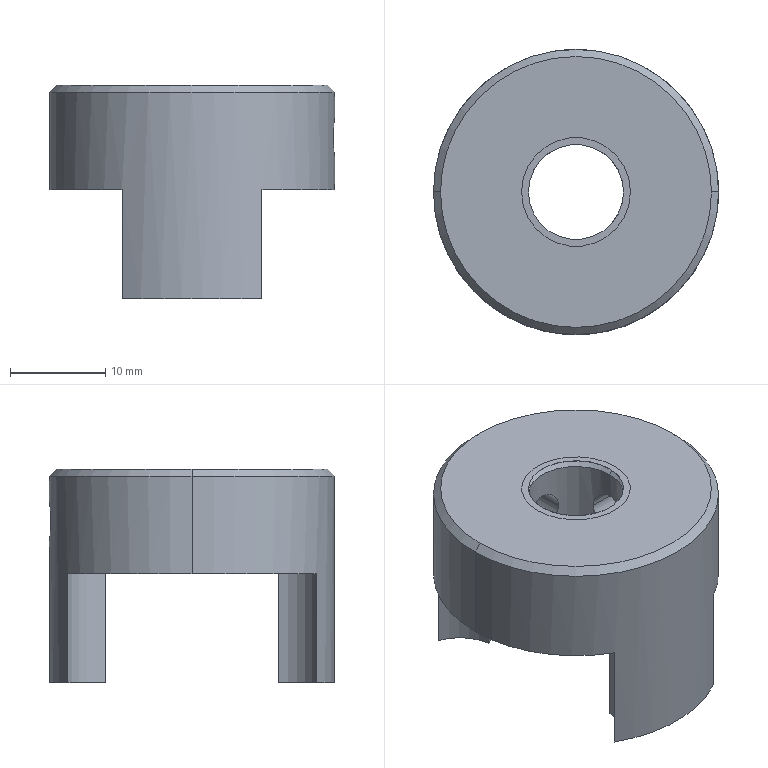Part | SolidWorks | features BaseBody 1 | 1 solid | 27 faces | box 30 x 30 x 22.5 mm | volume 7880 mm3 | cylinder 16 | cone 6 | plane 5 | commonest cylinder face diameters 10 x8 4 x4 19.8 x2 30 x2
STEP:
#1=CARTESIAN_POINT('',(0.,15.,10.));
#2=VERTEX_POINT('',#1);
#3=CARTESIAN_POINT('',(0.,15.,14.));
#4=VERTEX_POINT('',#3);
#5=CARTESIAN_POINT('',(0.,15.,10.));
#6=CARTESIAN_POINT('',(0.1323,15.,10.));
#7=CARTESIAN_POINT('',(0.2623,14.998,10.013));
#8=CARTESIAN_POINT('',(0.5181,14.992,10.064));
#9=CARTESIAN_POINT('',(0.6452,14.987,10.102));
#10=CARTESIAN_POINT('',(0.8873,14.974,10.203));
#11=CARTESIAN_POINT('',(1.002,14.967,10.264));
#12=CARTESIAN_POINT('',(1.219,14.951,10.409));
#13=CARTESIAN_POINT('',(1.322,14.942,10.494));
#14=CARTESIAN_POINT('',(1.599,14.916,10.77));
#15=CARTESIAN_POINT('',(1.747,14.898,10.993));
#16=CARTESIAN_POINT('',(1.947,14.873,11.474));
#17=CARTESIAN_POINT('',(2.,14.866,11.737));
#18=CARTESIAN_POINT('',(2.,14.866,12.129));
#19=CARTESIAN_POINT('',(1.987,14.868,12.262));
#20=CARTESIAN_POINT('',(1.936,14.875,12.518));
#21=CARTESIAN_POINT('',(1.898,14.879,12.643));
#22=CARTESIAN_POINT('',(1.798,14.892,12.885));
#23=CARTESIAN_POINT('',(1.736,14.899,13.002));
#24=CARTESIAN_POINT('',(1.591,14.916,13.219));
#25=CARTESIAN_POINT('',(1.508,14.924,13.32));
#26=CARTESIAN_POINT('',(1.322,14.942,13.507));
#27=CARTESIAN_POINT('',(1.221,14.951,13.589));
#28=CARTESIAN_POINT('',(1.005,14.967,13.734));
#29=CARTESIAN_POINT('',(0.8878,14.974,13.797));
#30=CARTESIAN_POINT('',(0.6458,14.987,13.897));
#31=CARTESIAN_POINT('',(0.5212,14.991,13.935));
#32=CARTESIAN_POINT('',(0.2647,14.998,13.987));
#33=CARTESIAN_POINT('',(0.1323,15.,14.));
#34=CARTESIAN_POINT('',(0.,15.,14.));
#35=B_SPLINE_CURVE_WITH_KNOTS('',3,(#5,#6,#7,#8,#9,#10,#11,#12,#13,#14,#15,#16,#17,#18,#19,#20,#21,#22,#23,#24,#25,#26,#27,#28,#29,#30,#31,#32,#33,#34),.UNSPECIFIED.,.F.,.F.,(4,2,2,2,2,2,2,2,2,2,2,2,2,2,4),(0.006258,0.00665,0.007041,0.007432,0.007823,0.008605,0.009388,0.009779,0.01017,0.01056,0.01095,0.01134,0.01173,0.01213,0.01252),.UNSPECIFIED.);
#36=EDGE_CURVE('',#2,#4,#35,.T.);
#37=ORIENTED_EDGE('',*,*,#36,.T.);
#38=CARTESIAN_POINT('',(0.,15.,14.));
#39=CARTESIAN_POINT('',(-0.1323,15.,14.));
#40=CARTESIAN_POINT('',(-0.2623,14.998,13.987));
#41=CARTESIAN_POINT('',(-0.5181,14.992,13.936));
#42=CARTESIAN_POINT('',(-0.6452,14.987,13.898));
#43=CARTESIAN_POINT('',(-0.8873,14.974,13.797));
#44=CARTESIAN_POINT('',(-1.002,14.967,13.736));
#45=CARTESIAN_POINT('',(-1.219,14.951,13.591));
#46=CARTESIAN_POINT('',(-1.322,14.942,13.506));
#47=CARTESIAN_POINT('',(-1.599,14.916,13.23));
#48=CARTESIAN_POINT('',(-1.747,14.898,13.007));
#49=CARTESIAN_POINT('',(-1.947,14.873,12.526));
#50=CARTESIAN_POINT('',(-2.,14.866,12.263));
#51=CARTESIAN_POINT('',(-2.,14.866,11.871));
#52=CARTESIAN_POINT('',(-1.987,14.868,11.738));
#53=CARTESIAN_POINT('',(-1.936,14.875,11.482));
#54=CARTESIAN_POINT('',(-1.898,14.879,11.357));
#55=CARTESIAN_POINT('',(-1.798,14.892,11.115));
#56=CARTESIAN_POINT('',(-1.736,14.899,10.998));
#57=CARTESIAN_POINT('',(-1.591,14.916,10.781));
#58=CARTESIAN_POINT('',(-1.508,14.924,10.68));
#59=CARTESIAN_POINT('',(-1.322,14.942,10.493));
#60=CARTESIAN_POINT('',(-1.221,14.951,10.411));
#61=CARTESIAN_POINT('',(-1.005,14.967,10.266));
#62=CARTESIAN_POINT('',(-0.8878,14.974,10.203));
#63=CARTESIAN_POINT('',(-0.6458,14.987,10.103));
#64=CARTESIAN_POINT('',(-0.5212,14.991,10.065));
#65=CARTESIAN_POINT('',(-0.2647,14.998,10.013));
#66=CARTESIAN_POINT('',(-0.1323,15.,10.));
#67=CARTESIAN_POINT('',(0.,15.,10.));
#68=B_SPLINE_CURVE_WITH_KNOTS('',3,(#38,#39,#40,#41,#42,#43,#44,#45,#46,#47,#48,#49,#50,#51,#52,#53,#54,#55,#56,#57,#58,#59,#60,#61,#62,#63,#64,#65,#66,#67),.UNSPECIFIED.,.F.,.F.,(4,2,2,2,2,2,2,2,2,2,2,2,2,2,4),(0.,0.0003912,0.0007823,0.001173,0.001565,0.002347,0.003129,0.00352,0.003912,0.004303,0.004694,0.005085,0.005476,0.005867,0.006258),.UNSPECIFIED.);
#69=EDGE_CURVE('',#4,#2,#68,.T.);
#70=ORIENTED_EDGE('',*,*,#69,.T.);
#71=EDGE_LOOP('',(#37,#70));
#72=FACE_BOUND('',#71,.T.);
#73=CARTESIAN_POINT('',(-15.,0.,16.75));
#74=VERTEX_POINT('',#73);
#75=CARTESIAN_POINT('',(15.,0.,16.75));
#76=VERTEX_POINT('',#75);
#77=CARTESIAN_POINT('',(0.,0.,16.75));
#78=DIRECTION('',(0.,0.,-1.));
#79=DIRECTION('',(-1.,0.,0.));
#80=AXIS2_PLACEMENT_3D('',#77,#78,#79);
#81=CIRCLE('',#80,15.);
#82=EDGE_CURVE('',#74,#76,#81,.T.);
#83=ORIENTED_EDGE('',*,*,#82,.T.);
#84=CARTESIAN_POINT('',(15.,0.,14.));
#85=VERTEX_POINT('',#84);
#86=CARTESIAN_POINT('',(15.,0.,11.625));
#87=DIRECTION('',(0.,0.,-1.));
#88=VECTOR('',#87,1000.);
#89=LINE('',#86,#88);
#90=EDGE_CURVE('',#76,#85,#89,.T.);
#91=ORIENTED_EDGE('',*,*,#90,.T.);
#92=CARTESIAN_POINT('',(14.866,2.,12.));
#93=VERTEX_POINT('',#92);
#94=CARTESIAN_POINT('',(15.,0.,14.));
#95=CARTESIAN_POINT('',(15.,0.1322,14.));
#96=CARTESIAN_POINT('',(14.998,0.2622,13.987));
#97=CARTESIAN_POINT('',(14.992,0.5179,13.936));
#98=CARTESIAN_POINT('',(14.987,0.6449,13.898));
#99=CARTESIAN_POINT('',(14.974,0.8869,13.797));
#100=CARTESIAN_POINT('',(14.967,1.002,13.736));
#101=CARTESIAN_POINT('',(14.951,1.219,13.591));
#102=CARTESIAN_POINT('',(14.942,1.322,13.507));
#103=CARTESIAN_POINT('',(14.916,1.598,13.231));
#104=CARTESIAN_POINT('',(14.898,1.747,13.008));
#105=CARTESIAN_POINT('',(14.873,1.947,12.527));
#106=CARTESIAN_POINT('',(14.866,2.,12.264));
#107=CARTESIAN_POINT('',(14.866,2.,12.));
#108=B_SPLINE_CURVE_WITH_KNOTS('',3,(#94,#95,#96,#97,#98,#99,#100,#101,#102,#103,#104,#105,#106,#107),.UNSPECIFIED.,.F.,.F.,(4,2,2,2,2,2,4),(0.006256,0.006647,0.007038,0.007429,0.00782,0.008602,0.009384),.UNSPECIFIED.);
#109=EDGE_CURVE('',#85,#93,#108,.T.);
#110=ORIENTED_EDGE('',*,*,#109,.T.);
#111=CARTESIAN_POINT('',(15.,0.,10.));
#112=VERTEX_POINT('',#111);
#113=CARTESIAN_POINT('',(14.866,2.,12.));
#114=CARTESIAN_POINT('',(14.866,2.,11.868));
#115=CARTESIAN_POINT('',(14.868,1.987,11.738));
#116=CARTESIAN_POINT('',(14.875,1.936,11.482));
#117=CARTESIAN_POINT('',(14.88,1.898,11.355));
#118=CARTESIAN_POINT('',(14.892,1.797,11.113));
#119=CARTESIAN_POINT('',(14.899,1.736,10.998));
#120=CARTESIAN_POINT('',(14.916,1.591,10.781));
#121=CARTESIAN_POINT('',(14.924,1.507,10.678));
#122=CARTESIAN_POINT('',(14.951,1.231,10.402));
#123=CARTESIAN_POINT('',(14.968,1.008,10.253));
#124=CARTESIAN_POINT('',(14.993,0.5271,10.053));
#125=CARTESIAN_POINT('',(15.,0.2644,10.));
#126=CARTESIAN_POINT('',(15.,0.,10.));
#127=B_SPLINE_CURVE_WITH_KNOTS('',3,(#113,#114,#115,#116,#117,#118,#119,#120,#121,#122,#123,#124,#125,#126),.UNSPECIFIED.,.F.,.F.,(4,2,2,2,2,2,4),(-0.003128,-0.002737,-0.002346,-0.001955,-0.001564,-0.0007819,0.),.UNSPECIFIED.);
#128=EDGE_CURVE('',#93,#112,#127,.T.);
#129=ORIENTED_EDGE('',*,*,#128,.T.);
#130=CARTESIAN_POINT('',(15.,0.,6.5));
#131=VERTEX_POINT('',#130);
#132=CARTESIAN_POINT('',(15.,0.,11.625));
#133=DIRECTION('',(0.,0.,-1.));
#134=VECTOR('',#133,1000.);
#135=LINE('',#132,#134);
#136=EDGE_CURVE('',#112,#131,#135,.T.);
#137=ORIENTED_EDGE('',*,*,#136,.T.);
#138=CARTESIAN_POINT('',(7.366,13.067,6.5));
#139=VERTEX_POINT('',#138);
#140=CARTESIAN_POINT('',(0.,0.,6.5));
#141=DIRECTION('',(0.,0.,1.));
#142=DIRECTION('',(-1.,0.,0.));
#143=AXIS2_PLACEMENT_3D('',#140,#141,#142);
#144=CIRCLE('',#143,15.);
#145=EDGE_CURVE('',#131,#139,#144,.T.);
#146=ORIENTED_EDGE('',*,*,#145,.T.);
#147=CARTESIAN_POINT('',(7.366,13.067,-5.));
#148=VERTEX_POINT('',#147);
#149=CARTESIAN_POINT('',(7.366,13.067,11.625));
#150=DIRECTION('',(0.,0.,-1.));
#151=VECTOR('',#150,1000.);
#152=LINE('',#149,#151);
#153=EDGE_CURVE('',#139,#148,#152,.T.);
#154=ORIENTED_EDGE('',*,*,#153,.T.);
#155=CARTESIAN_POINT('',(-7.366,13.067,-5.));
#156=VERTEX_POINT('',#155);
#157=CARTESIAN_POINT('',(0.,0.,-5.));
#158=DIRECTION('',(0.,0.,1.));
#159=DIRECTION('',(-1.,0.,0.));
#160=AXIS2_PLACEMENT_3D('',#157,#158,#159);
#161=CIRCLE('',#160,15.);
#162=EDGE_CURVE('',#148,#156,#161,.T.);
#163=ORIENTED_EDGE('',*,*,#162,.T.);
#164=CARTESIAN_POINT('',(-7.366,13.067,6.5));
#165=VERTEX_POINT('',#164);
#166=CARTESIAN_POINT('',(-7.366,13.067,11.625));
#167=DIRECTION('',(0.,0.,1.));
#168=VECTOR('',#167,1000.);
#169=LINE('',#166,#168);
#170=EDGE_CURVE('',#156,#165,#169,.T.);
#171=ORIENTED_EDGE('',*,*,#170,.T.);
#172=CARTESIAN_POINT('',(-15.,0.,6.5));
#173=VERTEX_POINT('',#172);
#174=CARTESIAN_POINT('',(0.,0.,6.5));
#175=DIRECTION('',(0.,0.,1.));
#176=DIRECTION('',(-1.,0.,0.));
#177=AXIS2_PLACEMENT_3D('',#174,#175,#176);
#178=CIRCLE('',#177,15.);
#179=EDGE_CURVE('',#165,#173,#178,.T.);
#180=ORIENTED_EDGE('',*,*,#179,.T.);
#181=CARTESIAN_POINT('',(-15.,0.,11.625));
#182=DIRECTION('',(0.,0.,-1.));
#183=VECTOR('',#182,1000.);
#184=LINE('',#181,#183);
#185=EDGE_CURVE('',#74,#173,#184,.T.);
#186=ORIENTED_EDGE('',*,*,#185,.F.);
#187=EDGE_LOOP('',(#83,#91,#110,#129,#137,#146,#154,#163,#171,#180,#186));
#188=FACE_OUTER_BOUND('',#187,.T.);
#189=CARTESIAN_POINT('',(0.,0.,11.625));
#190=DIRECTION('',(0.,0.,-1.));
#191=DIRECTION('',(-1.,0.,0.));
#192=AXIS2_PLACEMENT_3D('',#189,#190,#191);
#193=CYLINDRICAL_SURFACE('',#192,15.);
#194=ADVANCED_FACE('',(#72,#188),#193,.T.);
#195=ORIENTED_EDGE('',*,*,#128,.F.);
#196=CARTESIAN_POINT('',(4.583,2.,12.));
#197=VERTEX_POINT('',#196);
#198=CARTESIAN_POINT('',(7.5,2.,12.));
#199=DIRECTION('',(-1.,0.,0.));
#200=VECTOR('',#199,1000.);
#201=LINE('',#198,#200);
#202=EDGE_CURVE('',#93,#197,#201,.T.);
#203=ORIENTED_EDGE('',*,*,#202,.T.);
#204=CARTESIAN_POINT('',(5.,0.,10.));
#205=VERTEX_POINT('',#204);
#206=CARTESIAN_POINT('',(5.,0.,10.));
#207=CARTESIAN_POINT('',(5.,0.1336,10.));
#208=CARTESIAN_POINT('',(4.995,0.2647,10.013));
#209=CARTESIAN_POINT('',(4.974,0.5221,10.065));
#210=CARTESIAN_POINT('',(4.959,0.6499,10.104));
#211=CARTESIAN_POINT('',(4.921,0.8914,10.205));
#212=CARTESIAN_POINT('',(4.899,1.006,10.266));
#213=CARTESIAN_POINT('',(4.85,1.222,10.411));
#214=CARTESIAN_POINT('',(4.823,1.323,10.495));
#215=CARTESIAN_POINT('',(4.742,1.597,10.768));
#216=CARTESIAN_POINT('',(4.687,1.745,10.989));
#217=CARTESIAN_POINT('',(4.627,1.895,11.348));
#218=CARTESIAN_POINT('',(4.611,1.935,11.475));
#219=CARTESIAN_POINT('',(4.588,1.987,11.735));
#220=CARTESIAN_POINT('',(4.583,2.,11.866));
#221=CARTESIAN_POINT('',(4.583,2.,12.));
#222=B_SPLINE_CURVE_WITH_KNOTS('',3,(#206,#207,#208,#209,#210,#211,#212,#213,#214,#215,#216,#217,#218,#219,#220,#221),.UNSPECIFIED.,.F.,.F.,(4,2,2,2,2,2,2,4),(0.006316,0.006711,0.007106,0.0075,0.007895,0.008684,0.009079,0.009474),.UNSPECIFIED.);
#223=EDGE_CURVE('',#205,#197,#222,.T.);
#224=ORIENTED_EDGE('',*,*,#223,.F.);
#225=CARTESIAN_POINT('',(4.583,-2.,12.));
#226=VERTEX_POINT('',#225);
#227=CARTESIAN_POINT('',(4.583,-2.,12.));
#228=CARTESIAN_POINT('',(4.583,-2.,11.866));
#229=CARTESIAN_POINT('',(4.588,-1.987,11.735));
#230=CARTESIAN_POINT('',(4.61,-1.935,11.478));
#231=CARTESIAN_POINT('',(4.627,-1.896,11.35));
#232=CARTESIAN_POINT('',(4.667,-1.795,11.109));
#233=CARTESIAN_POINT('',(4.69,-1.734,10.995));
#234=CARTESIAN_POINT('',(4.741,-1.589,10.779));
#235=CARTESIAN_POINT('',(4.769,-1.506,10.678));
#236=CARTESIAN_POINT('',(4.849,-1.233,10.404));
#237=CARTESIAN_POINT('',(4.903,-1.012,10.255));
#238=CARTESIAN_POINT('',(4.959,-0.6519,10.105));
#239=CARTESIAN_POINT('',(4.974,-0.5246,10.066));
#240=CARTESIAN_POINT('',(4.995,-0.2652,10.013));
#241=CARTESIAN_POINT('',(5.,-0.1336,10.));
#242=CARTESIAN_POINT('',(5.,0.,10.));
#243=B_SPLINE_CURVE_WITH_KNOTS('',3,(#227,#228,#229,#230,#231,#232,#233,#234,#235,#236,#237,#238,#239,#240,#241,#242),.UNSPECIFIED.,.F.,.F.,(4,2,2,2,2,2,2,4),(0.003158,0.003553,0.003948,0.004342,0.004737,0.005527,0.005921,0.006316),.UNSPECIFIED.);
#244=EDGE_CURVE('',#226,#205,#243,.T.);
#245=ORIENTED_EDGE('',*,*,#244,.F.);
#246=CARTESIAN_POINT('',(14.866,-2.,12.));
#247=VERTEX_POINT('',#246);
#248=CARTESIAN_POINT('',(7.5,-2.,12.));
#249=DIRECTION('',(-1.,0.,0.));
#250=VECTOR('',#249,1000.);
#251=LINE('',#248,#250);
#252=EDGE_CURVE('',#247,#226,#251,.T.);
#253=ORIENTED_EDGE('',*,*,#252,.F.);
#254=CARTESIAN_POINT('',(15.,0.,10.));
#255=CARTESIAN_POINT('',(15.,-0.1322,10.));
#256=CARTESIAN_POINT('',(14.998,-0.2622,10.013));
#257=CARTESIAN_POINT('',(14.992,-0.5179,10.064));
#258=CARTESIAN_POINT('',(14.987,-0.6449,10.102));
#259=CARTESIAN_POINT('',(14.974,-0.8869,10.203));
#260=CARTESIAN_POINT('',(14.967,-1.002,10.264));
#261=CARTESIAN_POINT('',(14.951,-1.219,10.409));
#262=CARTESIAN_POINT('',(14.942,-1.322,10.493));
#263=CARTESIAN_POINT('',(14.916,-1.598,10.769));
#264=CARTESIAN_POINT('',(14.898,-1.747,10.992));
#265=CARTESIAN_POINT('',(14.873,-1.947,11.473));
#266=CARTESIAN_POINT('',(14.866,-2.,11.736));
#267=CARTESIAN_POINT('',(14.866,-2.,12.));
#268=B_SPLINE_CURVE_WITH_KNOTS('',3,(#254,#255,#256,#257,#258,#259,#260,#261,#262,#263,#264,#265,#266,#267),.UNSPECIFIED.,.F.,.F.,(4,2,2,2,2,2,4),(0.,0.000391,0.0007819,0.001173,0.001564,0.002346,0.003128),.UNSPECIFIED.);
#269=EDGE_CURVE('',#112,#247,#268,.T.);
#270=ORIENTED_EDGE('',*,*,#269,.F.);
#271=EDGE_LOOP('',(#195,#203,#224,#245,#253,#270));
#272=FACE_OUTER_BOUND('',#271,.T.);
#273=CARTESIAN_POINT('',(7.5,0.,12.));
#274=DIRECTION('',(-1.,0.,0.));
#275=DIRECTION('',(0.,-1.,0.));
#276=AXIS2_PLACEMENT_3D('',#273,#274,#275);
#277=CYLINDRICAL_SURFACE('',#276,2.);
#278=ADVANCED_FACE('',(#272),#277,.F.);
#279=CARTESIAN_POINT('',(-14.25,0.,17.5));
#280=VERTEX_POINT('',#279);
#281=CARTESIAN_POINT('',(14.25,0.,17.5));
#282=VERTEX_POINT('',#281);
#283=CARTESIAN_POINT('',(0.,0.,17.5));
#284=DIRECTION('',(0.,0.,-1.));
#285=DIRECTION('',(-1.,0.,0.));
#286=AXIS2_PLACEMENT_3D('',#283,#284,#285);
#287=CIRCLE('',#286,14.25);
#288=EDGE_CURVE('',#280,#282,#287,.T.);
#289=ORIENTED_EDGE('',*,*,#288,.T.);
#290=CARTESIAN_POINT('',(15.,0.,16.75));
#291=DIRECTION('',(0.7071,0.,-0.7071));
#292=VECTOR('',#291,1000.);
#293=LINE('',#290,#292);
#294=EDGE_CURVE('',#282,#76,#293,.T.);
#295=ORIENTED_EDGE('',*,*,#294,.T.);
#296=ORIENTED_EDGE('',*,*,#82,.F.);
#297=CARTESIAN_POINT('',(-15.,0.,16.75));
#298=DIRECTION('',(-0.7071,0.,-0.7071));
#299=VECTOR('',#298,1000.);
#300=LINE('',#297,#299);
#301=EDGE_CURVE('',#280,#74,#300,.T.);
#302=ORIENTED_EDGE('',*,*,#301,.F.);
#303=EDGE_LOOP('',(#289,#295,#296,#302));
#304=FACE_OUTER_BOUND('',#303,.T.);
#305=CARTESIAN_POINT('',(0.,0.,16.75));
#306=DIRECTION('',(0.,0.,-1.));
#307=DIRECTION('',(-1.,0.,0.));
#308=AXIS2_PLACEMENT_3D('',#305,#306,#307);
#309=CONICAL_SURFACE('',#308,15.,0.7854);
#310=ADVANCED_FACE('',(#304),#309,.T.);
#311=CARTESIAN_POINT('',(5.,0.,16.75));
#312=VERTEX_POINT('',#311);
#313=CARTESIAN_POINT('',(-5.,0.,16.75));
#314=VERTEX_POINT('',#313);
#315=CARTESIAN_POINT('',(0.,0.,16.75));
#316=DIRECTION('',(0.,0.,-1.));
#317=DIRECTION('',(-1.,0.,0.));
#318=AXIS2_PLACEMENT_3D('',#315,#316,#317);
#319=CIRCLE('',#318,5.);
#320=EDGE_CURVE('',#312,#314,#319,.T.);
#321=ORIENTED_EDGE('',*,*,#320,.F.);
#322=CARTESIAN_POINT('',(5.,0.,14.));
#323=VERTEX_POINT('',#322);
#324=CARTESIAN_POINT('',(5.,0.,12.));
#325=DIRECTION('',(0.,0.,-1.));
#326=VECTOR('',#325,1000.);
#327=LINE('',#324,#326);
#328=EDGE_CURVE('',#312,#323,#327,.T.);
#329=ORIENTED_EDGE('',*,*,#328,.T.);
#330=CARTESIAN_POINT('',(5.,0.,14.));
#331=CARTESIAN_POINT('',(5.,-0.1336,14.));
#332=CARTESIAN_POINT('',(4.995,-0.2647,13.987));
#333=CARTESIAN_POINT('',(4.974,-0.5221,13.935));
#334=CARTESIAN_POINT('',(4.959,-0.6499,13.896));
#335=CARTESIAN_POINT('',(4.921,-0.8914,13.795));
#336=CARTESIAN_POINT('',(4.899,-1.006,13.734));
#337=CARTESIAN_POINT('',(4.85,-1.222,13.589));
#338=CARTESIAN_POINT('',(4.823,-1.323,13.505));
#339=CARTESIAN_POINT('',(4.742,-1.597,13.232));
#340=CARTESIAN_POINT('',(4.687,-1.745,13.011));
#341=CARTESIAN_POINT('',(4.627,-1.895,12.652));
#342=CARTESIAN_POINT('',(4.611,-1.935,12.525));
#343=CARTESIAN_POINT('',(4.588,-1.987,12.265));
#344=CARTESIAN_POINT('',(4.583,-2.,12.134));
#345=CARTESIAN_POINT('',(4.583,-2.,12.));
#346=B_SPLINE_CURVE_WITH_KNOTS('',3,(#330,#331,#332,#333,#334,#335,#336,#337,#338,#339,#340,#341,#342,#343,#344,#345),.UNSPECIFIED.,.F.,.F.,(4,2,2,2,2,2,2,4),(0.,0.0003948,0.0007895,0.001184,0.001579,0.002369,0.002763,0.003158),.UNSPECIFIED.);
#347=EDGE_CURVE('',#323,#226,#346,.T.);
#348=ORIENTED_EDGE('',*,*,#347,.T.);
#349=ORIENTED_EDGE('',*,*,#244,.T.);
#350=CARTESIAN_POINT('',(5.,0.,7.25));
#351=VERTEX_POINT('',#350);
#352=CARTESIAN_POINT('',(5.,0.,12.));
#353=DIRECTION('',(0.,0.,-1.));
#354=VECTOR('',#353,1000.);
#355=LINE('',#352,#354);
#356=EDGE_CURVE('',#205,#351,#355,.T.);
#357=ORIENTED_EDGE('',*,*,#356,.T.);
#358=CARTESIAN_POINT('',(-5.,0.,7.25));
#359=VERTEX_POINT('',#358);
#360=CARTESIAN_POINT('',(0.,0.,7.25));
#361=DIRECTION('',(0.,0.,1.));
#362=DIRECTION('',(-1.,0.,0.));
#363=AXIS2_PLACEMENT_3D('',#360,#361,#362);
#364=CIRCLE('',#363,5.);
#365=EDGE_CURVE('',#359,#351,#364,.T.);
#366=ORIENTED_EDGE('',*,*,#365,.F.);
#367=CARTESIAN_POINT('',(-5.,0.,12.));
#368=DIRECTION('',(0.,0.,-1.));
#369=VECTOR('',#368,1000.);
#370=LINE('',#367,#369);
#371=EDGE_CURVE('',#314,#359,#370,.T.);
#372=ORIENTED_EDGE('',*,*,#371,.F.);
#373=EDGE_LOOP('',(#321,#329,#348,#349,#357,#366,#372));
#374=FACE_OUTER_BOUND('',#373,.T.);
#375=CARTESIAN_POINT('',(0.,0.,12.));
#376=DIRECTION('',(0.,0.,-1.));
#377=DIRECTION('',(-1.,0.,0.));
#378=AXIS2_PLACEMENT_3D('',#375,#376,#377);
#379=CYLINDRICAL_SURFACE('',#378,5.);
#380=ADVANCED_FACE('',(#374),#379,.F.);
#381=ORIENTED_EDGE('',*,*,#69,.F.);
#382=CARTESIAN_POINT('',(0.,5.,14.));
#383=VERTEX_POINT('',#382);
#384=CARTESIAN_POINT('',(0.,7.5,14.));
#385=DIRECTION('',(0.,-1.,0.));
#386=VECTOR('',#385,1000.);
#387=LINE('',#384,#386);
#388=EDGE_CURVE('',#4,#383,#387,.T.);
#389=ORIENTED_EDGE('',*,*,#388,.T.);
#390=CARTESIAN_POINT('',(0.,5.,10.));
#391=VERTEX_POINT('',#390);
#392=CARTESIAN_POINT('',(0.,5.,14.));
#393=CARTESIAN_POINT('',(-0.1336,5.,14.));
#394=CARTESIAN_POINT('',(-0.2647,4.995,13.987));
#395=CARTESIAN_POINT('',(-0.5222,4.974,13.935));
#396=CARTESIAN_POINT('',(-0.6499,4.959,13.896));
#397=CARTESIAN_POINT('',(-0.8916,4.921,13.795));
#398=CARTESIAN_POINT('',(-1.006,4.899,13.734));
#399=CARTESIAN_POINT('',(-1.222,4.85,13.588));
#400=CARTESIAN_POINT('',(-1.323,4.823,13.505));
#401=CARTESIAN_POINT('',(-1.597,4.742,13.231));
#402=CARTESIAN_POINT('',(-1.745,4.687,13.011));
#403=CARTESIAN_POINT('',(-1.895,4.627,12.651));
#404=CARTESIAN_POINT('',(-1.935,4.611,12.524));
#405=CARTESIAN_POINT('',(-1.987,4.588,12.265));
#406=CARTESIAN_POINT('',(-2.,4.583,12.135));
#407=CARTESIAN_POINT('',(-2.,4.583,11.871));
#408=CARTESIAN_POINT('',(-1.987,4.588,11.737));
#409=CARTESIAN_POINT('',(-1.935,4.61,11.479));
#410=CARTESIAN_POINT('',(-1.897,4.626,11.353));
#411=CARTESIAN_POINT('',(-1.796,4.667,11.11));
#412=CARTESIAN_POINT('',(-1.734,4.69,10.995));
#413=CARTESIAN_POINT('',(-1.59,4.741,10.78));
#414=CARTESIAN_POINT('',(-1.507,4.769,10.678));
#415=CARTESIAN_POINT('',(-1.324,4.823,10.495));
#416=CARTESIAN_POINT('',(-1.224,4.849,10.413));
#417=CARTESIAN_POINT('',(-1.008,4.899,10.268));
#418=CARTESIAN_POINT('',(-0.8919,4.921,10.205));
#419=CARTESIAN_POINT('',(-0.5316,4.978,10.054));
#420=CARTESIAN_POINT('',(-0.2673,5.,10.));
#421=CARTESIAN_POINT('',(0.,5.,10.));
#422=B_SPLINE_CURVE_WITH_KNOTS('',3,(#392,#393,#394,#395,#396,#397,#398,#399,#400,#401,#402,#403,#404,#405,#406,#407,#408,#409,#410,#411,#412,#413,#414,#415,#416,#417,#418,#419,#420,#421),.UNSPECIFIED.,.F.,.F.,(4,2,2,2,2,2,2,2,2,2,2,2,2,2,4),(0.,0.0003948,0.0007896,0.001184,0.001579,0.002369,0.002764,0.003158,0.003553,0.003948,0.004343,0.004738,0.005133,0.005527,0.006317),.UNSPECIFIED.);
#423=EDGE_CURVE('',#383,#391,#422,.T.);
#424=ORIENTED_EDGE('',*,*,#423,.T.);
#425=CARTESIAN_POINT('',(0.,7.5,10.));
#426=DIRECTION('',(0.,-1.,0.));
#427=VECTOR('',#426,1000.);
#428=LINE('',#425,#427);
#429=EDGE_CURVE('',#2,#391,#428,.T.);
#430=ORIENTED_EDGE('',*,*,#429,.F.);
#431=EDGE_LOOP('',(#381,#389,#424,#430));
#432=FACE_OUTER_BOUND('',#431,.T.);
#433=CARTESIAN_POINT('',(0.,7.5,12.));
#434=DIRECTION('',(0.,-1.,0.));
#435=DIRECTION('',(0.,0.,-1.));
#436=AXIS2_PLACEMENT_3D('',#433,#434,#435);
#437=CYLINDRICAL_SURFACE('',#436,2.);
#438=ADVANCED_FACE('',(#432),#437,.F.);
#439=ORIENTED_EDGE('',*,*,#365,.T.);
#440=CARTESIAN_POINT('',(5.75,0.,6.5));
#441=VERTEX_POINT('',#440);
#442=CARTESIAN_POINT('',(5.75,0.,6.5));
#443=DIRECTION('',(0.7071,0.,-0.7071));
#444=VECTOR('',#443,1000.);
#445=LINE('',#442,#444);
#446=EDGE_CURVE('',#351,#441,#445,.T.);
#447=ORIENTED_EDGE('',*,*,#446,.T.);
#448=CARTESIAN_POINT('',(-5.75,0.,6.5));
#449=VERTEX_POINT('',#448);
#450=CARTESIAN_POINT('',(0.,0.,6.5));
#451=DIRECTION('',(0.,0.,1.));
#452=DIRECTION('',(-1.,0.,0.));
#453=AXIS2_PLACEMENT_3D('',#450,#451,#452);
#454=CIRCLE('',#453,5.75);
#455=EDGE_CURVE('',#449,#441,#454,.T.);
#456=ORIENTED_EDGE('',*,*,#455,.F.);
#457=CARTESIAN_POINT('',(-5.75,0.,6.5));
#458=DIRECTION('',(-0.7071,0.,-0.7071));
#459=VECTOR('',#458,1000.);
#460=LINE('',#457,#459);
#461=EDGE_CURVE('',#359,#449,#460,.T.);
#462=ORIENTED_EDGE('',*,*,#461,.F.);
#463=EDGE_LOOP('',(#439,#447,#456,#462));
#464=FACE_OUTER_BOUND('',#463,.T.);
#465=CARTESIAN_POINT('',(0.,0.,6.5));
#466=DIRECTION('',(0.,0.,-1.));
#467=DIRECTION('',(-1.,0.,0.));
#468=AXIS2_PLACEMENT_3D('',#465,#466,#467);
#469=CONICAL_SURFACE('',#468,5.75,0.7854);
#470=ADVANCED_FACE('',(#464),#469,.F.);
#471=ORIENTED_EDGE('',*,*,#320,.T.);
#472=CARTESIAN_POINT('',(-5.73,0.,17.48));
#473=VERTEX_POINT('',#472);
#474=CARTESIAN_POINT('',(-5.73,0.,17.48));
#475=DIRECTION('',(-0.7071,0.,0.7071));
#476=VECTOR('',#475,1000.);
#477=LINE('',#474,#476);
#478=EDGE_CURVE('',#314,#473,#477,.T.);
#479=ORIENTED_EDGE('',*,*,#478,.T.);
#480=CARTESIAN_POINT('',(5.73,0.,17.48));
#481=VERTEX_POINT('',#480);
#482=CARTESIAN_POINT('',(0.,0.,17.48));
#483=DIRECTION('',(0.,0.,-1.));
#484=DIRECTION('',(1.,0.,0.));
#485=AXIS2_PLACEMENT_3D('',#482,#483,#484);
#486=CIRCLE('',#485,5.73);
#487=EDGE_CURVE('',#481,#473,#486,.T.);
#488=ORIENTED_EDGE('',*,*,#487,.F.);
#489=CARTESIAN_POINT('',(5.73,0.,17.48));
#490=DIRECTION('',(0.7071,0.,0.7071));
#491=VECTOR('',#490,1000.);
#492=LINE('',#489,#491);
#493=EDGE_CURVE('',#312,#481,#492,.T.);
#494=ORIENTED_EDGE('',*,*,#493,.F.);
#495=EDGE_LOOP('',(#471,#479,#488,#494));
#496=FACE_OUTER_BOUND('',#495,.T.);
#497=CARTESIAN_POINT('',(0.,0.,17.48));
#498=DIRECTION('',(0.,0.,1.));
#499=DIRECTION('',(1.,0.,0.));
#500=AXIS2_PLACEMENT_3D('',#497,#498,#499);
#501=CONICAL_SURFACE('',#500,5.73,0.7854);
#502=ADVANCED_FACE('',(#496),#501,.F.);
#503=CARTESIAN_POINT('',(-5.,0.,17.48));
#504=VERTEX_POINT('',#503);
#505=CARTESIAN_POINT('',(5.,0.,17.48));
#506=VERTEX_POINT('',#505);
#507=CARTESIAN_POINT('',(0.,0.,17.48));
#508=DIRECTION('',(0.,0.,1.));
#509=DIRECTION('',(1.,0.,0.));
#510=AXIS2_PLACEMENT_3D('',#507,#508,#509);
#511=CIRCLE('',#510,5.);
#512=EDGE_CURVE('',#504,#506,#511,.T.);
#513=ORIENTED_EDGE('',*,*,#512,.F.);
#514=CARTESIAN_POINT('',(-5.,0.,17.5));
#515=VERTEX_POINT('',#514);
#516=CARTESIAN_POINT('',(-5.,0.,-5.));
#517=DIRECTION('',(0.,0.,1.));
#518=VECTOR('',#517,1000.);
#519=LINE('',#516,#518);
#520=EDGE_CURVE('',#504,#515,#519,.T.);
#521=ORIENTED_EDGE('',*,*,#520,.T.);
#522=CARTESIAN_POINT('',(5.,0.,17.5));
#523=VERTEX_POINT('',#522);
#524=CARTESIAN_POINT('',(0.,0.,17.5));
#525=DIRECTION('',(0.,0.,-1.));
#526=DIRECTION('',(1.,0.,0.));
#527=AXIS2_PLACEMENT_3D('',#524,#525,#526);
#528=CIRCLE('',#527,5.);
#529=EDGE_CURVE('',#523,#515,#528,.T.);
#530=ORIENTED_EDGE('',*,*,#529,.F.);
#531=CARTESIAN_POINT('',(5.,0.,-5.));
#532=DIRECTION('',(0.,0.,1.));
#533=VECTOR('',#532,1000.);
#534=LINE('',#531,#533);
#535=EDGE_CURVE('',#506,#523,#534,.T.);
#536=ORIENTED_EDGE('',*,*,#535,.F.);
#537=EDGE_LOOP('',(#513,#521,#530,#536));
#538=FACE_OUTER_BOUND('',#537,.T.);
#539=CARTESIAN_POINT('',(0.,0.,-5.));
#540=DIRECTION('',(0.,0.,1.));
#541=DIRECTION('',(1.,0.,0.));
#542=AXIS2_PLACEMENT_3D('',#539,#540,#541);
#543=CYLINDRICAL_SURFACE('',#542,5.);
#544=ADVANCED_FACE('',(#538),#543,.F.);
#545=ORIENTED_EDGE('',*,*,#90,.F.);
#546=CARTESIAN_POINT('',(0.,0.,16.75));
#547=DIRECTION('',(0.,0.,-1.));
#548=DIRECTION('',(-1.,0.,0.));
#549=AXIS2_PLACEMENT_3D('',#546,#547,#548);
#550=CIRCLE('',#549,15.);
#551=EDGE_CURVE('',#76,#74,#550,.T.);
#552=ORIENTED_EDGE('',*,*,#551,.T.);
#553=ORIENTED_EDGE('',*,*,#185,.T.);
#554=CARTESIAN_POINT('',(-7.366,-13.067,6.5));
#555=VERTEX_POINT('',#554);
#556=CARTESIAN_POINT('',(0.,0.,6.5));
#557=DIRECTION('',(0.,0.,1.));
#558=DIRECTION('',(-1.,0.,0.));
#559=AXIS2_PLACEMENT_3D('',#556,#557,#558);
#560=CIRCLE('',#559,15.);
#561=EDGE_CURVE('',#173,#555,#560,.T.);
#562=ORIENTED_EDGE('',*,*,#561,.T.);
#563=CARTESIAN_POINT('',(-7.366,-13.067,-5.));
#564=VERTEX_POINT('',#563);
#565=CARTESIAN_POINT('',(-7.366,-13.067,11.625));
#566=DIRECTION('',(0.,0.,-1.));
#567=VECTOR('',#566,1000.);
#568=LINE('',#565,#567);
#569=EDGE_CURVE('',#555,#564,#568,.T.);
#570=ORIENTED_EDGE('',*,*,#569,.T.);
#571=CARTESIAN_POINT('',(7.366,-13.067,-5.));
#572=VERTEX_POINT('',#571);
#573=CARTESIAN_POINT('',(0.,0.,-5.));
#574=DIRECTION('',(0.,0.,1.));
#575=DIRECTION('',(-1.,0.,0.));
#576=AXIS2_PLACEMENT_3D('',#573,#574,#575);
#577=CIRCLE('',#576,15.);
#578=EDGE_CURVE('',#564,#572,#577,.T.);
#579=ORIENTED_EDGE('',*,*,#578,.T.);
#580=CARTESIAN_POINT('',(7.366,-13.067,6.5));
#581=VERTEX_POINT('',#580);
#582=CARTESIAN_POINT('',(7.366,-13.067,11.625));
#583=DIRECTION('',(0.,0.,1.));
#584=VECTOR('',#583,1000.);
#585=LINE('',#582,#584);
#586=EDGE_CURVE('',#572,#581,#585,.T.);
#587=ORIENTED_EDGE('',*,*,#586,.T.);
#588=CARTESIAN_POINT('',(0.,0.,6.5));
#589=DIRECTION('',(0.,0.,1.));
#590=DIRECTION('',(-1.,0.,0.));
#591=AXIS2_PLACEMENT_3D('',#588,#589,#590);
#592=CIRCLE('',#591,15.);
#593=EDGE_CURVE('',#581,#131,#592,.T.);
#594=ORIENTED_EDGE('',*,*,#593,.T.);
#595=ORIENTED_EDGE('',*,*,#136,.F.);
#596=ORIENTED_EDGE('',*,*,#269,.T.);
#597=CARTESIAN_POINT('',(14.866,-2.,12.));
#598=CARTESIAN_POINT('',(14.866,-2.,12.132));
#599=CARTESIAN_POINT('',(14.868,-1.987,12.262));
#600=CARTESIAN_POINT('',(14.875,-1.936,12.518));
#601=CARTESIAN_POINT('',(14.88,-1.898,12.645));
#602=CARTESIAN_POINT('',(14.892,-1.797,12.887));
#603=CARTESIAN_POINT('',(14.899,-1.736,13.002));
#604=CARTESIAN_POINT('',(14.916,-1.591,13.219));
#605=CARTESIAN_POINT('',(14.924,-1.507,13.322));
#606=CARTESIAN_POINT('',(14.951,-1.231,13.598));
#607=CARTESIAN_POINT('',(14.968,-1.008,13.747));
#608=CARTESIAN_POINT('',(14.993,-0.5271,13.947));
#609=CARTESIAN_POINT('',(15.,-0.2644,14.));
#610=CARTESIAN_POINT('',(15.,0.,14.));
#611=B_SPLINE_CURVE_WITH_KNOTS('',3,(#597,#598,#599,#600,#601,#602,#603,#604,#605,#606,#607,#608,#609,#610),.UNSPECIFIED.,.F.,.F.,(4,2,2,2,2,2,4),(0.003128,0.003519,0.00391,0.004301,0.004692,0.005474,0.006256),.UNSPECIFIED.);
#612=EDGE_CURVE('',#247,#85,#611,.T.);
#613=ORIENTED_EDGE('',*,*,#612,.T.);
#614=EDGE_LOOP('',(#545,#552,#553,#562,#570,#579,#587,#594,#595,#596,#613));
#615=FACE_OUTER_BOUND('',#614,.T.);
#616=CARTESIAN_POINT('',(0.,0.,11.625));
#617=DIRECTION('',(0.,0.,-1.));
#618=DIRECTION('',(-1.,0.,0.));
#619=AXIS2_PLACEMENT_3D('',#616,#617,#618);
#620=CYLINDRICAL_SURFACE('',#619,15.);
#621=ADVANCED_FACE('',(#615),#620,.T.);
#622=ORIENTED_EDGE('',*,*,#202,.F.);
#623=ORIENTED_EDGE('',*,*,#109,.F.);
#624=ORIENTED_EDGE('',*,*,#612,.F.);
#625=ORIENTED_EDGE('',*,*,#252,.T.);
#626=ORIENTED_EDGE('',*,*,#347,.F.);
#627=CARTESIAN_POINT('',(4.583,2.,12.));
#628=CARTESIAN_POINT('',(4.583,2.,12.134));
#629=CARTESIAN_POINT('',(4.588,1.987,12.265));
#630=CARTESIAN_POINT('',(4.61,1.935,12.522));
#631=CARTESIAN_POINT('',(4.627,1.896,12.65));
#632=CARTESIAN_POINT('',(4.667,1.795,12.891));
#633=CARTESIAN_POINT('',(4.69,1.734,13.005));
#634=CARTESIAN_POINT('',(4.741,1.589,13.221));
#635=CARTESIAN_POINT('',(4.769,1.506,13.322));
#636=CARTESIAN_POINT('',(4.849,1.233,13.596));
#637=CARTESIAN_POINT('',(4.903,1.012,13.745));
#638=CARTESIAN_POINT('',(4.959,0.6519,13.895));
#639=CARTESIAN_POINT('',(4.974,0.5246,13.934));
#640=CARTESIAN_POINT('',(4.995,0.2652,13.987));
#641=CARTESIAN_POINT('',(5.,0.1336,14.));
#642=CARTESIAN_POINT('',(5.,0.,14.));
#643=B_SPLINE_CURVE_WITH_KNOTS('',3,(#627,#628,#629,#630,#631,#632,#633,#634,#635,#636,#637,#638,#639,#640,#641,#642),.UNSPECIFIED.,.F.,.F.,(4,2,2,2,2,2,2,4),(-0.003158,-0.002763,-0.002369,-0.001974,-0.001579,-0.0007895,-0.0003948,0.),.UNSPECIFIED.);
#644=EDGE_CURVE('',#197,#323,#643,.T.);
#645=ORIENTED_EDGE('',*,*,#644,.F.);
#646=EDGE_LOOP('',(#622,#623,#624,#625,#626,#645));
#647=FACE_OUTER_BOUND('',#646,.T.);
#648=CARTESIAN_POINT('',(7.5,0.,12.));
#649=DIRECTION('',(-1.,0.,0.));
#650=DIRECTION('',(0.,-1.,0.));
#651=AXIS2_PLACEMENT_3D('',#648,#649,#650);
#652=CYLINDRICAL_SURFACE('',#651,2.);
#653=ADVANCED_FACE('',(#647),#652,.F.);
#654=ORIENTED_EDGE('',*,*,#179,.F.);
#655=CARTESIAN_POINT('',(-4.,9.056,6.5));
#656=VERTEX_POINT('',#655);
#657=CARTESIAN_POINT('',(-8.946,8.323,6.5));
#658=DIRECTION('',(0.,0.,-1.));
#659=DIRECTION('',(-1.,0.,0.));
#660=AXIS2_PLACEMENT_3D('',#657,#658,#659);
#661=CIRCLE('',#660,5.);
#662=EDGE_CURVE('',#165,#656,#661,.T.);
#663=ORIENTED_EDGE('',*,*,#662,.T.);
#664=CARTESIAN_POINT('',(4.,9.056,6.5));
#665=VERTEX_POINT('',#664);
#666=CARTESIAN_POINT('',(0.,0.,6.5));
#667=DIRECTION('',(0.,0.,-1.));
#668=DIRECTION('',(-1.,0.,0.));
#669=AXIS2_PLACEMENT_3D('',#666,#667,#668);
#670=CIRCLE('',#669,9.9);
#671=EDGE_CURVE('',#656,#665,#670,.T.);
#672=ORIENTED_EDGE('',*,*,#671,.T.);
#673=CARTESIAN_POINT('',(8.946,8.323,6.5));
#674=DIRECTION('',(0.,0.,-1.));
#675=DIRECTION('',(-1.,0.,0.));
#676=AXIS2_PLACEMENT_3D('',#673,#674,#675);
#677=CIRCLE('',#676,5.);
#678=EDGE_CURVE('',#665,#139,#677,.T.);
#679=ORIENTED_EDGE('',*,*,#678,.T.);
#680=ORIENTED_EDGE('',*,*,#145,.F.);
#681=ORIENTED_EDGE('',*,*,#593,.F.);
#682=CARTESIAN_POINT('',(4.,-9.056,6.5));
#683=VERTEX_POINT('',#682);
#684=CARTESIAN_POINT('',(8.946,-8.323,6.5));
#685=DIRECTION('',(0.,0.,-1.));
#686=DIRECTION('',(-1.,0.,0.));
#687=AXIS2_PLACEMENT_3D('',#684,#685,#686);
#688=CIRCLE('',#687,5.);
#689=EDGE_CURVE('',#581,#683,#688,.T.);
#690=ORIENTED_EDGE('',*,*,#689,.T.);
#691=CARTESIAN_POINT('',(-4.,-9.056,6.5));
#692=VERTEX_POINT('',#691);
#693=CARTESIAN_POINT('',(0.,0.,6.5));
#694=DIRECTION('',(0.,0.,-1.));
#695=DIRECTION('',(-1.,0.,0.));
#696=AXIS2_PLACEMENT_3D('',#693,#694,#695);
#697=CIRCLE('',#696,9.9);
#698=EDGE_CURVE('',#683,#692,#697,.T.);
#699=ORIENTED_EDGE('',*,*,#698,.T.);
#700=CARTESIAN_POINT('',(-8.946,-8.323,6.5));
#701=DIRECTION('',(0.,0.,-1.));
#702=DIRECTION('',(-1.,0.,0.));
#703=AXIS2_PLACEMENT_3D('',#700,#701,#702);
#704=CIRCLE('',#703,5.);
#705=EDGE_CURVE('',#692,#555,#704,.T.);
#706=ORIENTED_EDGE('',*,*,#705,.T.);
#707=ORIENTED_EDGE('',*,*,#561,.F.);
#708=EDGE_LOOP('',(#654,#663,#672,#679,#680,#681,#690,#699,#706,#707));
#709=FACE_OUTER_BOUND('',#708,.T.);
#710=ORIENTED_EDGE('',*,*,#455,.T.);
#711=CARTESIAN_POINT('',(0.,0.,6.5));
#712=DIRECTION('',(0.,0.,1.));
#713=DIRECTION('',(-1.,0.,0.));
#714=AXIS2_PLACEMENT_3D('',#711,#712,#713);
#715=CIRCLE('',#714,5.75);
#716=EDGE_CURVE('',#441,#449,#715,.T.);
#717=ORIENTED_EDGE('',*,*,#716,.T.);
#718=EDGE_LOOP('',(#710,#717));
#719=FACE_BOUND('',#718,.T.);
#720=CARTESIAN_POINT('',(0.,10.375,6.5));
#721=DIRECTION('',(0.,0.,-1.));
#722=DIRECTION('',(-1.,0.,0.));
#723=AXIS2_PLACEMENT_3D('',#720,#721,#722);
#724=PLANE('',#723);
#725=ADVANCED_FACE('',(#709,#719),#724,.T.);
#726=ORIENTED_EDGE('',*,*,#689,.F.);
#727=ORIENTED_EDGE('',*,*,#586,.F.);
#728=CARTESIAN_POINT('',(4.,-9.056,-5.));
#729=VERTEX_POINT('',#728);
#730=CARTESIAN_POINT('',(8.946,-8.323,-5.));
#731=DIRECTION('',(0.,0.,1.));
#732=DIRECTION('',(-1.,0.,0.));
#733=AXIS2_PLACEMENT_3D('',#730,#731,#732);
#734=CIRCLE('',#733,5.);
#735=EDGE_CURVE('',#729,#572,#734,.T.);
#736=ORIENTED_EDGE('',*,*,#735,.F.);
#737=CARTESIAN_POINT('',(4.,-9.056,6.5));
#738=DIRECTION('',(0.,0.,-1.));
#739=VECTOR('',#738,1000.);
#740=LINE('',#737,#739);
#741=EDGE_CURVE('',#683,#729,#740,.T.);
#742=ORIENTED_EDGE('',*,*,#741,.F.);
#743=EDGE_LOOP('',(#726,#727,#736,#742));
#744=FACE_OUTER_BOUND('',#743,.T.);
#745=CARTESIAN_POINT('',(8.946,-8.323,6.5));
#746=DIRECTION('',(0.,0.,-1.));
#747=DIRECTION('',(-1.,0.,0.));
#748=AXIS2_PLACEMENT_3D('',#745,#746,#747);
#749=CYLINDRICAL_SURFACE('',#748,5.);
#750=ADVANCED_FACE('',(#744),#749,.F.);
#751=ORIENTED_EDGE('',*,*,#578,.F.);
#752=CARTESIAN_POINT('',(-4.,-9.056,-5.));
#753=VERTEX_POINT('',#752);
#754=CARTESIAN_POINT('',(-8.946,-8.323,-5.));
#755=DIRECTION('',(0.,0.,-1.));
#756=DIRECTION('',(-1.,0.,0.));
#757=AXIS2_PLACEMENT_3D('',#754,#755,#756);
#758=CIRCLE('',#757,5.);
#759=EDGE_CURVE('',#753,#564,#758,.T.);
#760=ORIENTED_EDGE('',*,*,#759,.F.);
#761=CARTESIAN_POINT('',(0.,0.,-5.));
#762=DIRECTION('',(0.,0.,-1.));
#763=DIRECTION('',(-1.,0.,0.));
#764=AXIS2_PLACEMENT_3D('',#761,#762,#763);
#765=CIRCLE('',#764,9.9);
#766=EDGE_CURVE('',#729,#753,#765,.T.);
#767=ORIENTED_EDGE('',*,*,#766,.F.);
#768=ORIENTED_EDGE('',*,*,#735,.T.);
#769=EDGE_LOOP('',(#751,#760,#767,#768));
#770=FACE_OUTER_BOUND('',#769,.T.);
#771=CARTESIAN_POINT('',(0.000000001,-12.2,-5.));
#772=DIRECTION('',(0.,0.,1.));
#773=DIRECTION('',(0.,-1.,0.));
#774=AXIS2_PLACEMENT_3D('',#771,#772,#773);
#775=PLANE('',#774);
#776=ADVANCED_FACE('',(#770),#775,.F.);
#777=ORIENTED_EDGE('',*,*,#705,.F.);
#778=CARTESIAN_POINT('',(-4.,-9.056,6.5));
#779=DIRECTION('',(0.,0.,1.));
#780=VECTOR('',#779,1000.);
#781=LINE('',#778,#780);
#782=EDGE_CURVE('',#753,#692,#781,.T.);
#783=ORIENTED_EDGE('',*,*,#782,.F.);
#784=ORIENTED_EDGE('',*,*,#759,.T.);
#785=ORIENTED_EDGE('',*,*,#569,.F.);
#786=EDGE_LOOP('',(#777,#783,#784,#785));
#787=FACE_OUTER_BOUND('',#786,.T.);
#788=CARTESIAN_POINT('',(-8.946,-8.323,6.5));
#789=DIRECTION('',(0.,0.,-1.));
#790=DIRECTION('',(-1.,0.,0.));
#791=AXIS2_PLACEMENT_3D('',#788,#789,#790);
#792=CYLINDRICAL_SURFACE('',#791,5.);
#793=ADVANCED_FACE('',(#787),#792,.F.);
#794=ORIENTED_EDGE('',*,*,#294,.F.);
#795=CARTESIAN_POINT('',(0.,0.,17.5));
#796=DIRECTION('',(0.,0.,-1.));
#797=DIRECTION('',(-1.,0.,0.));
#798=AXIS2_PLACEMENT_3D('',#795,#796,#797);
#799=CIRCLE('',#798,14.25);
#800=EDGE_CURVE('',#282,#280,#799,.T.);
#801=ORIENTED_EDGE('',*,*,#800,.T.);
#802=ORIENTED_EDGE('',*,*,#301,.T.);
#803=ORIENTED_EDGE('',*,*,#551,.F.);
#804=EDGE_LOOP('',(#794,#801,#802,#803));
#805=FACE_OUTER_BOUND('',#804,.T.);
#806=CARTESIAN_POINT('',(0.,0.,16.75));
#807=DIRECTION('',(0.,0.,-1.));
#808=DIRECTION('',(-1.,0.,0.));
#809=AXIS2_PLACEMENT_3D('',#806,#807,#808);
#810=CONICAL_SURFACE('',#809,15.,0.7854);
#811=ADVANCED_FACE('',(#805),#810,.T.);
#812=ORIENTED_EDGE('',*,*,#328,.F.);
#813=CARTESIAN_POINT('',(0.,0.,16.75));
#814=DIRECTION('',(0.,0.,-1.));
#815=DIRECTION('',(-1.,0.,0.));
#816=AXIS2_PLACEMENT_3D('',#813,#814,#815);
#817=CIRCLE('',#816,5.);
#818=EDGE_CURVE('',#314,#312,#817,.T.);
#819=ORIENTED_EDGE('',*,*,#818,.F.);
#820=ORIENTED_EDGE('',*,*,#371,.T.);
#821=CARTESIAN_POINT('',(0.,0.,7.25));
#822=DIRECTION('',(0.,0.,1.));
#823=DIRECTION('',(-1.,0.,0.));
#824=AXIS2_PLACEMENT_3D('',#821,#822,#823);
#825=CIRCLE('',#824,5.);
#826=EDGE_CURVE('',#351,#359,#825,.T.);
#827=ORIENTED_EDGE('',*,*,#826,.F.);
#828=ORIENTED_EDGE('',*,*,#356,.F.);
#829=ORIENTED_EDGE('',*,*,#223,.T.);
#830=ORIENTED_EDGE('',*,*,#644,.T.);
#831=EDGE_LOOP('',(#812,#819,#820,#827,#828,#829,#830));
#832=FACE_OUTER_BOUND('',#831,.T.);
#833=CARTESIAN_POINT('',(0.,5.,10.));
#834=CARTESIAN_POINT('',(0.1336,5.,10.));
#835=CARTESIAN_POINT('',(0.2647,4.995,10.013));
#836=CARTESIAN_POINT('',(0.5222,4.974,10.065));
#837=CARTESIAN_POINT('',(0.6499,4.959,10.104));
#838=CARTESIAN_POINT('',(0.8916,4.921,10.205));
#839=CARTESIAN_POINT('',(1.006,4.899,10.266));
#840=CARTESIAN_POINT('',(1.222,4.85,10.412));
#841=CARTESIAN_POINT('',(1.323,4.823,10.495));
#842=CARTESIAN_POINT('',(1.597,4.742,10.769));
#843=CARTESIAN_POINT('',(1.745,4.687,10.989));
#844=CARTESIAN_POINT('',(1.895,4.627,11.349));
#845=CARTESIAN_POINT('',(1.935,4.611,11.476));
#846=CARTESIAN_POINT('',(1.987,4.588,11.735));
#847=CARTESIAN_POINT('',(2.,4.583,11.865));
#848=CARTESIAN_POINT('',(2.,4.583,12.129));
#849=CARTESIAN_POINT('',(1.987,4.588,12.263));
#850=CARTESIAN_POINT('',(1.935,4.61,12.521));
#851=CARTESIAN_POINT('',(1.897,4.626,12.647));
#852=CARTESIAN_POINT('',(1.796,4.667,12.89));
#853=CARTESIAN_POINT('',(1.734,4.69,13.005));
#854=CARTESIAN_POINT('',(1.59,4.741,13.22));
#855=CARTESIAN_POINT('',(1.507,4.769,13.322));
#856=CARTESIAN_POINT('',(1.324,4.823,13.505));
#857=CARTESIAN_POINT('',(1.224,4.849,13.587));
#858=CARTESIAN_POINT('',(1.008,4.899,13.732));
#859=CARTESIAN_POINT('',(0.8919,4.921,13.795));
#860=CARTESIAN_POINT('',(0.5316,4.978,13.946));
#861=CARTESIAN_POINT('',(0.2671,5.,14.));
#862=CARTESIAN_POINT('',(0.,5.,14.));
#863=B_SPLINE_CURVE_WITH_KNOTS('',3,(#833,#834,#835,#836,#837,#838,#839,#840,#841,#842,#843,#844,#845,#846,#847,#848,#849,#850,#851,#852,#853,#854,#855,#856,#857,#858,#859,#860,#861,#862),.UNSPECIFIED.,.F.,.F.,(4,2,2,2,2,2,2,2,2,2,2,2,2,2,4),(0.006317,0.006712,0.007106,0.007501,0.007896,0.008685,0.00908,0.009474,0.009869,0.01026,0.01066,0.01105,0.01145,0.01184,0.01263),.UNSPECIFIED.);
#864=EDGE_CURVE('',#391,#383,#863,.T.);
#865=ORIENTED_EDGE('',*,*,#864,.F.);
#866=ORIENTED_EDGE('',*,*,#423,.F.);
#867=EDGE_LOOP('',(#865,#866));
#868=FACE_BOUND('',#867,.T.);
#869=CARTESIAN_POINT('',(0.,0.,12.));
#870=DIRECTION('',(0.,0.,-1.));
#871=DIRECTION('',(-1.,0.,0.));
#872=AXIS2_PLACEMENT_3D('',#869,#870,#871);
#873=CYLINDRICAL_SURFACE('',#872,5.);
#874=ADVANCED_FACE('',(#832,#868),#873,.F.);
#875=ORIENTED_EDGE('',*,*,#662,.F.);
#876=ORIENTED_EDGE('',*,*,#170,.F.);
#877=CARTESIAN_POINT('',(-4.,9.056,-5.));
#878=VERTEX_POINT('',#877);
#879=CARTESIAN_POINT('',(-8.946,8.323,-5.));
#880=DIRECTION('',(0.,0.,1.));
#881=DIRECTION('',(-1.,0.,0.));
#882=AXIS2_PLACEMENT_3D('',#879,#880,#881);
#883=CIRCLE('',#882,5.);
#884=EDGE_CURVE('',#878,#156,#883,.T.);
#885=ORIENTED_EDGE('',*,*,#884,.F.);
#886=CARTESIAN_POINT('',(-4.,9.056,6.5));
#887=DIRECTION('',(0.,0.,-1.));
#888=VECTOR('',#887,1000.);
#889=LINE('',#886,#888);
#890=EDGE_CURVE('',#656,#878,#889,.T.);
#891=ORIENTED_EDGE('',*,*,#890,.F.);
#892=EDGE_LOOP('',(#875,#876,#885,#891));
#893=FACE_OUTER_BOUND('',#892,.T.);
#894=CARTESIAN_POINT('',(-8.946,8.323,6.5));
#895=DIRECTION('',(0.,0.,-1.));
#896=DIRECTION('',(-1.,0.,0.));
#897=AXIS2_PLACEMENT_3D('',#894,#895,#896);
#898=CYLINDRICAL_SURFACE('',#897,5.);
#899=ADVANCED_FACE('',(#893),#898,.F.);
#900=CARTESIAN_POINT('',(4.,9.056,-5.));
#901=VERTEX_POINT('',#900);
#902=CARTESIAN_POINT('',(8.946,8.323,-5.));
#903=DIRECTION('',(0.,0.,-1.));
#904=DIRECTION('',(-1.,0.,0.));
#905=AXIS2_PLACEMENT_3D('',#902,#903,#904);
#906=CIRCLE('',#905,5.);
#907=EDGE_CURVE('',#901,#148,#906,.T.);
#908=ORIENTED_EDGE('',*,*,#907,.F.);
#909=CARTESIAN_POINT('',(0.,0.,-5.));
#910=DIRECTION('',(0.,0.,-1.));
#911=DIRECTION('',(-1.,0.,0.));
#912=AXIS2_PLACEMENT_3D('',#909,#910,#911);
#913=CIRCLE('',#912,9.9);
#914=EDGE_CURVE('',#878,#901,#913,.T.);
#915=ORIENTED_EDGE('',*,*,#914,.F.);
#916=ORIENTED_EDGE('',*,*,#884,.T.);
#917=ORIENTED_EDGE('',*,*,#162,.F.);
#918=EDGE_LOOP('',(#908,#915,#916,#917));
#919=FACE_OUTER_BOUND('',#918,.T.);
#920=CARTESIAN_POINT('',(-0.000000001,12.2,-5.));
#921=DIRECTION('',(0.,0.,1.));
#922=DIRECTION('',(0.,-1.,0.));
#923=AXIS2_PLACEMENT_3D('',#920,#921,#922);
#924=PLANE('',#923);
#925=ADVANCED_FACE('',(#919),#924,.F.);
#926=ORIENTED_EDGE('',*,*,#678,.F.);
#927=CARTESIAN_POINT('',(4.,9.056,6.5));
#928=DIRECTION('',(0.,0.,1.));
#929=VECTOR('',#928,1000.);
#930=LINE('',#927,#929);
#931=EDGE_CURVE('',#901,#665,#930,.T.);
#932=ORIENTED_EDGE('',*,*,#931,.F.);
#933=ORIENTED_EDGE('',*,*,#907,.T.);
#934=ORIENTED_EDGE('',*,*,#153,.F.);
#935=EDGE_LOOP('',(#926,#932,#933,#934));
#936=FACE_OUTER_BOUND('',#935,.T.);
#937=CARTESIAN_POINT('',(8.946,8.323,6.5));
#938=DIRECTION('',(0.,0.,-1.));
#939=DIRECTION('',(-1.,0.,0.));
#940=AXIS2_PLACEMENT_3D('',#937,#938,#939);
#941=CYLINDRICAL_SURFACE('',#940,5.);
#942=ADVANCED_FACE('',(#936),#941,.F.);
#943=ORIENTED_EDGE('',*,*,#388,.F.);
#944=ORIENTED_EDGE('',*,*,#36,.F.);
#945=ORIENTED_EDGE('',*,*,#429,.T.);
#946=ORIENTED_EDGE('',*,*,#864,.T.);
#947=EDGE_LOOP('',(#943,#944,#945,#946));
#948=FACE_OUTER_BOUND('',#947,.T.);
#949=CARTESIAN_POINT('',(0.,7.5,12.));
#950=DIRECTION('',(0.,-1.,0.));
#951=DIRECTION('',(0.,0.,-1.));
#952=AXIS2_PLACEMENT_3D('',#949,#950,#951);
#953=CYLINDRICAL_SURFACE('',#952,2.);
#954=ADVANCED_FACE('',(#948),#953,.F.);
#955=ORIENTED_EDGE('',*,*,#698,.F.);
#956=ORIENTED_EDGE('',*,*,#741,.T.);
#957=ORIENTED_EDGE('',*,*,#766,.T.);
#958=ORIENTED_EDGE('',*,*,#782,.T.);
#959=EDGE_LOOP('',(#955,#956,#957,#958));
#960=FACE_OUTER_BOUND('',#959,.T.);
#961=CARTESIAN_POINT('',(0.,0.,6.5));
#962=DIRECTION('',(0.,0.,-1.));
#963=DIRECTION('',(-1.,0.,0.));
#964=AXIS2_PLACEMENT_3D('',#961,#962,#963);
#965=CYLINDRICAL_SURFACE('',#964,9.9);
#966=ADVANCED_FACE('',(#960),#965,.F.);
#967=ORIENTED_EDGE('',*,*,#671,.F.);
#968=ORIENTED_EDGE('',*,*,#890,.T.);
#969=ORIENTED_EDGE('',*,*,#914,.T.);
#970=ORIENTED_EDGE('',*,*,#931,.T.);
#971=EDGE_LOOP('',(#967,#968,#969,#970));
#972=FACE_OUTER_BOUND('',#971,.T.);
#973=CARTESIAN_POINT('',(0.,0.,6.5));
#974=DIRECTION('',(0.,0.,-1.));
#975=DIRECTION('',(-1.,0.,0.));
#976=AXIS2_PLACEMENT_3D('',#973,#974,#975);
#977=CYLINDRICAL_SURFACE('',#976,9.9);
#978=ADVANCED_FACE('',(#972),#977,.F.);
#979=ORIENTED_EDGE('',*,*,#446,.F.);
#980=ORIENTED_EDGE('',*,*,#826,.T.);
#981=ORIENTED_EDGE('',*,*,#461,.T.);
#982=ORIENTED_EDGE('',*,*,#716,.F.);
#983=EDGE_LOOP('',(#979,#980,#981,#982));
#984=FACE_OUTER_BOUND('',#983,.T.);
#985=CARTESIAN_POINT('',(0.,0.,6.5));
#986=DIRECTION('',(0.,0.,-1.));
#987=DIRECTION('',(-1.,0.,0.));
#988=AXIS2_PLACEMENT_3D('',#985,#986,#987);
#989=CONICAL_SURFACE('',#988,5.75,0.7854);
#990=ADVANCED_FACE('',(#984),#989,.F.);
#991=ORIENTED_EDGE('',*,*,#288,.F.);
#992=ORIENTED_EDGE('',*,*,#800,.F.);
#993=EDGE_LOOP('',(#991,#992));
#994=FACE_OUTER_BOUND('',#993,.T.);
#995=ORIENTED_EDGE('',*,*,#529,.T.);
#996=CARTESIAN_POINT('',(0.,0.,17.5));
#997=DIRECTION('',(0.,0.,-1.));
#998=DIRECTION('',(1.,0.,0.));
#999=AXIS2_PLACEMENT_3D('',#996,#997,#998);
#1000=CIRCLE('',#999,5.);
#1001=EDGE_CURVE('',#515,#523,#1000,.T.);
#1002=ORIENTED_EDGE('',*,*,#1001,.T.);
#1003=EDGE_LOOP('',(#995,#1002));
#1004=FACE_BOUND('',#1003,.T.);
#1005=CARTESIAN_POINT('',(0.,10.,17.5));
#1006=DIRECTION('',(0.,0.,1.));
#1007=DIRECTION('',(1.,0.,0.));
#1008=AXIS2_PLACEMENT_3D('',#1005,#1006,#1007);
#1009=PLANE('',#1008);
#1010=ADVANCED_FACE('',(#994,#1004),#1009,.T.);
#1011=ORIENTED_EDGE('',*,*,#478,.F.);
#1012=ORIENTED_EDGE('',*,*,#818,.T.);
#1013=ORIENTED_EDGE('',*,*,#493,.T.);
#1014=CARTESIAN_POINT('',(0.,0.,17.48));
#1015=DIRECTION('',(0.,0.,-1.));
#1016=DIRECTION('',(1.,0.,0.));
#1017=AXIS2_PLACEMENT_3D('',#1014,#1015,#1016);
#1018=CIRCLE('',#1017,5.73);
#1019=EDGE_CURVE('',#473,#481,#1018,.T.);
#1020=ORIENTED_EDGE('',*,*,#1019,.F.);
#1021=EDGE_LOOP('',(#1011,#1012,#1013,#1020));
#1022=FACE_OUTER_BOUND('',#1021,.T.);
#1023=CARTESIAN_POINT('',(0.,0.,17.48));
#1024=DIRECTION('',(0.,0.,1.));
#1025=DIRECTION('',(1.,0.,0.));
#1026=AXIS2_PLACEMENT_3D('',#1023,#1024,#1025);
#1027=CONICAL_SURFACE('',#1026,5.73,0.7854);
#1028=ADVANCED_FACE('',(#1022),#1027,.F.);
#1029=ORIENTED_EDGE('',*,*,#520,.F.);
#1030=CARTESIAN_POINT('',(0.,0.,17.48));
#1031=DIRECTION('',(0.,0.,1.));
#1032=DIRECTION('',(1.,0.,0.));
#1033=AXIS2_PLACEMENT_3D('',#1030,#1031,#1032);
#1034=CIRCLE('',#1033,5.);
#1035=EDGE_CURVE('',#506,#504,#1034,.T.);
#1036=ORIENTED_EDGE('',*,*,#1035,.F.);
#1037=ORIENTED_EDGE('',*,*,#535,.T.);
#1038=ORIENTED_EDGE('',*,*,#1001,.F.);
#1039=EDGE_LOOP('',(#1029,#1036,#1037,#1038));
#1040=FACE_OUTER_BOUND('',#1039,.T.);
#1041=CARTESIAN_POINT('',(0.,0.,-5.));
#1042=DIRECTION('',(0.,0.,1.));
#1043=DIRECTION('',(1.,0.,0.));
#1044=AXIS2_PLACEMENT_3D('',#1041,#1042,#1043);
#1045=CYLINDRICAL_SURFACE('',#1044,5.);
#1046=ADVANCED_FACE('',(#1040),#1045,.F.);
#1047=ORIENTED_EDGE('',*,*,#487,.T.);
#1048=ORIENTED_EDGE('',*,*,#1019,.T.);
#1049=EDGE_LOOP('',(#1047,#1048));
#1050=FACE_OUTER_BOUND('',#1049,.T.);
#1051=ORIENTED_EDGE('',*,*,#1035,.T.);
#1052=ORIENTED_EDGE('',*,*,#512,.T.);
#1053=EDGE_LOOP('',(#1051,#1052));
#1054=FACE_BOUND('',#1053,.T.);
#1055=CARTESIAN_POINT('',(0.,0.,17.48));
#1056=DIRECTION('',(0.,0.,1.));
#1057=DIRECTION('',(1.,0.,0.));
#1058=AXIS2_PLACEMENT_3D('',#1055,#1056,#1057);
#1059=PLANE('',#1058);
#1060=ADVANCED_FACE('',(#1050,#1054),#1059,.F.);
#1061=CLOSED_SHELL('',(#194,#278,#310,#380,#438,#470,#502,#544,#621,#653,#725,#750,#776,#793,#811,#874,#899,#925,#942,#954,#966,#978,#990,#1010,#1028,#1046,#1060));
#1062=MANIFOLD_SOLID_BREP('',#1061);
#1063=CARTESIAN_POINT('',(0.,0.,0.));
#1064=DIRECTION('',(0.,0.,1.));
#1065=DIRECTION('',(1.,0.,0.));
#1066=AXIS2_PLACEMENT_3D('',#1063,#1064,#1065);
#1067=(LENGTH_UNIT()NAMED_UNIT(*)SI_UNIT(.MILLI.,.METRE.));
#1068=UNCERTAINTY_MEASURE_WITH_UNIT(LENGTH_MEASURE(0.00001),#1067,'','');
#1069=(NAMED_UNIT(*)PLANE_ANGLE_UNIT()SI_UNIT($,.RADIAN.));
#1070=(NAMED_UNIT(*)SI_UNIT($,.STERADIAN.)SOLID_ANGLE_UNIT());
#1071=(GEOMETRIC_REPRESENTATION_CONTEXT(3)GLOBAL_UNCERTAINTY_ASSIGNED_CONTEXT((#1068))GLOBAL_UNIT_ASSIGNED_CONTEXT((#1067,#1069,#1070))REPRESENTATION_CONTEXT('',''));
#1072=ADVANCED_BREP_SHAPE_REPRESENTATION('',(#1062,#1066),#1071);